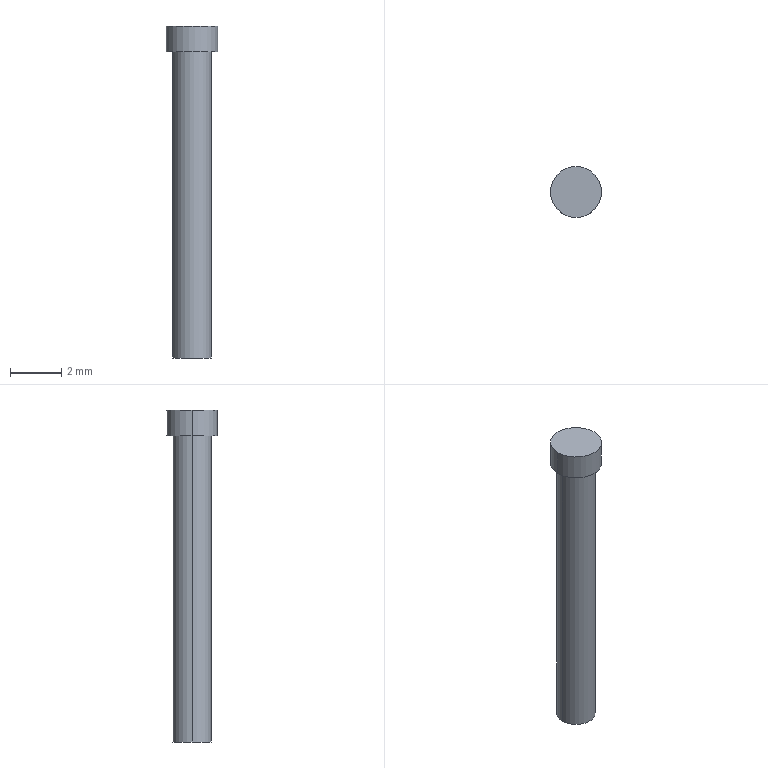Part | SolidWorks | features Extrusion 1, ICE 1 | 1 solid | 7 faces | box 2 x 2 x 13 mm | volume 24.347 mm3 | cylinder 4 | plane 3 | commonest cylinder face diameters 1.5 x2 2 x2
STEP:
#1=CARTESIAN_POINT('',(1.,0.,13.));
#2=VERTEX_POINT('',#1);
#3=CARTESIAN_POINT('',(-1.,0.,13.));
#4=VERTEX_POINT('',#3);
#5=CARTESIAN_POINT('',(0.,0.,13.));
#6=DIRECTION('',(0.,0.,1.));
#7=DIRECTION('',(1.,0.,0.));
#8=AXIS2_PLACEMENT_3D('',#5,#6,#7);
#9=CIRCLE('',#8,1.);
#10=EDGE_CURVE('',#2,#4,#9,.T.);
#11=ORIENTED_EDGE('',*,*,#10,.F.);
#12=CARTESIAN_POINT('',(1.,0.,12.));
#13=VERTEX_POINT('',#12);
#14=CARTESIAN_POINT('',(1.,0.,13.));
#15=DIRECTION('',(0.,0.,-1.));
#16=VECTOR('',#15,1000.);
#17=LINE('',#14,#16);
#18=EDGE_CURVE('',#2,#13,#17,.T.);
#19=ORIENTED_EDGE('',*,*,#18,.T.);
#20=CARTESIAN_POINT('',(-1.,0.,12.));
#21=VERTEX_POINT('',#20);
#22=CARTESIAN_POINT('',(0.,0.,12.));
#23=DIRECTION('',(0.,0.,1.));
#24=DIRECTION('',(1.,0.,0.));
#25=AXIS2_PLACEMENT_3D('',#22,#23,#24);
#26=CIRCLE('',#25,1.);
#27=EDGE_CURVE('',#13,#21,#26,.T.);
#28=ORIENTED_EDGE('',*,*,#27,.T.);
#29=CARTESIAN_POINT('',(-1.,0.,13.));
#30=DIRECTION('',(0.,0.,-1.));
#31=VECTOR('',#30,1000.);
#32=LINE('',#29,#31);
#33=EDGE_CURVE('',#4,#21,#32,.T.);
#34=ORIENTED_EDGE('',*,*,#33,.F.);
#35=EDGE_LOOP('',(#11,#19,#28,#34));
#36=FACE_OUTER_BOUND('',#35,.T.);
#37=CARTESIAN_POINT('',(0.,0.,13.));
#38=DIRECTION('',(0.,0.,-1.));
#39=DIRECTION('',(-1.,0.,0.));
#40=AXIS2_PLACEMENT_3D('',#37,#38,#39);
#41=CYLINDRICAL_SURFACE('',#40,1.);
#42=ADVANCED_FACE('',(#36),#41,.T.);
#43=CARTESIAN_POINT('',(0.75,0.,12.));
#44=VERTEX_POINT('',#43);
#45=CARTESIAN_POINT('',(-0.75,0.,12.));
#46=VERTEX_POINT('',#45);
#47=CARTESIAN_POINT('',(0.,0.,12.));
#48=DIRECTION('',(0.,0.,1.));
#49=DIRECTION('',(1.,0.,0.));
#50=AXIS2_PLACEMENT_3D('',#47,#48,#49);
#51=CIRCLE('',#50,0.75);
#52=EDGE_CURVE('',#44,#46,#51,.T.);
#53=ORIENTED_EDGE('',*,*,#52,.F.);
#54=CARTESIAN_POINT('',(0.75,0.,0.));
#55=VERTEX_POINT('',#54);
#56=CARTESIAN_POINT('',(0.75,0.,12.));
#57=DIRECTION('',(0.,0.,-1.));
#58=VECTOR('',#57,1000.);
#59=LINE('',#56,#58);
#60=EDGE_CURVE('',#44,#55,#59,.T.);
#61=ORIENTED_EDGE('',*,*,#60,.T.);
#62=CARTESIAN_POINT('',(-0.75,0.,0.));
#63=VERTEX_POINT('',#62);
#64=CARTESIAN_POINT('',(0.,0.,0.));
#65=DIRECTION('',(0.,0.,1.));
#66=DIRECTION('',(1.,0.,0.));
#67=AXIS2_PLACEMENT_3D('',#64,#65,#66);
#68=CIRCLE('',#67,0.75);
#69=EDGE_CURVE('',#55,#63,#68,.T.);
#70=ORIENTED_EDGE('',*,*,#69,.T.);
#71=CARTESIAN_POINT('',(-0.75,0.,12.));
#72=DIRECTION('',(0.,0.,-1.));
#73=VECTOR('',#72,1000.);
#74=LINE('',#71,#73);
#75=EDGE_CURVE('',#46,#63,#74,.T.);
#76=ORIENTED_EDGE('',*,*,#75,.F.);
#77=EDGE_LOOP('',(#53,#61,#70,#76));
#78=FACE_OUTER_BOUND('',#77,.T.);
#79=CARTESIAN_POINT('',(0.,0.,12.));
#80=DIRECTION('',(0.,0.,-1.));
#81=DIRECTION('',(-1.,0.,0.));
#82=AXIS2_PLACEMENT_3D('',#79,#80,#81);
#83=CYLINDRICAL_SURFACE('',#82,0.75);
#84=ADVANCED_FACE('',(#78),#83,.T.);
#85=ORIENTED_EDGE('',*,*,#60,.F.);
#86=CARTESIAN_POINT('',(0.,0.,12.));
#87=DIRECTION('',(0.,0.,1.));
#88=DIRECTION('',(1.,0.,0.));
#89=AXIS2_PLACEMENT_3D('',#86,#87,#88);
#90=CIRCLE('',#89,0.75);
#91=EDGE_CURVE('',#46,#44,#90,.T.);
#92=ORIENTED_EDGE('',*,*,#91,.F.);
#93=ORIENTED_EDGE('',*,*,#75,.T.);
#94=CARTESIAN_POINT('',(0.,0.,0.));
#95=DIRECTION('',(0.,0.,1.));
#96=DIRECTION('',(1.,0.,0.));
#97=AXIS2_PLACEMENT_3D('',#94,#95,#96);
#98=CIRCLE('',#97,0.75);
#99=EDGE_CURVE('',#63,#55,#98,.T.);
#100=ORIENTED_EDGE('',*,*,#99,.T.);
#101=EDGE_LOOP('',(#85,#92,#93,#100));
#102=FACE_OUTER_BOUND('',#101,.T.);
#103=CARTESIAN_POINT('',(0.,0.,12.));
#104=DIRECTION('',(0.,0.,-1.));
#105=DIRECTION('',(-1.,0.,0.));
#106=AXIS2_PLACEMENT_3D('',#103,#104,#105);
#107=CYLINDRICAL_SURFACE('',#106,0.75);
#108=ADVANCED_FACE('',(#102),#107,.T.);
#109=ORIENTED_EDGE('',*,*,#99,.F.);
#110=ORIENTED_EDGE('',*,*,#69,.F.);
#111=EDGE_LOOP('',(#109,#110));
#112=FACE_OUTER_BOUND('',#111,.T.);
#113=CARTESIAN_POINT('',(0.,0.,0.));
#114=DIRECTION('',(0.,0.,1.));
#115=DIRECTION('',(1.,0.,0.));
#116=AXIS2_PLACEMENT_3D('',#113,#114,#115);
#117=PLANE('',#116);
#118=ADVANCED_FACE('',(#112),#117,.F.);
#119=ORIENTED_EDGE('',*,*,#18,.F.);
#120=CARTESIAN_POINT('',(0.,0.,13.));
#121=DIRECTION('',(0.,0.,1.));
#122=DIRECTION('',(1.,0.,0.));
#123=AXIS2_PLACEMENT_3D('',#120,#121,#122);
#124=CIRCLE('',#123,1.);
#125=EDGE_CURVE('',#4,#2,#124,.T.);
#126=ORIENTED_EDGE('',*,*,#125,.F.);
#127=ORIENTED_EDGE('',*,*,#33,.T.);
#128=CARTESIAN_POINT('',(0.,0.,12.));
#129=DIRECTION('',(0.,0.,1.));
#130=DIRECTION('',(1.,0.,0.));
#131=AXIS2_PLACEMENT_3D('',#128,#129,#130);
#132=CIRCLE('',#131,1.);
#133=EDGE_CURVE('',#21,#13,#132,.T.);
#134=ORIENTED_EDGE('',*,*,#133,.T.);
#135=EDGE_LOOP('',(#119,#126,#127,#134));
#136=FACE_OUTER_BOUND('',#135,.T.);
#137=CARTESIAN_POINT('',(0.,0.,13.));
#138=DIRECTION('',(0.,0.,-1.));
#139=DIRECTION('',(-1.,0.,0.));
#140=AXIS2_PLACEMENT_3D('',#137,#138,#139);
#141=CYLINDRICAL_SURFACE('',#140,1.);
#142=ADVANCED_FACE('',(#136),#141,.T.);
#143=ORIENTED_EDGE('',*,*,#125,.T.);
#144=ORIENTED_EDGE('',*,*,#10,.T.);
#145=EDGE_LOOP('',(#143,#144));
#146=FACE_OUTER_BOUND('',#145,.T.);
#147=CARTESIAN_POINT('',(0.,0.,13.));
#148=DIRECTION('',(0.,0.,1.));
#149=DIRECTION('',(1.,0.,0.));
#150=AXIS2_PLACEMENT_3D('',#147,#148,#149);
#151=PLANE('',#150);
#152=ADVANCED_FACE('',(#146),#151,.T.);
#153=ORIENTED_EDGE('',*,*,#91,.T.);
#154=ORIENTED_EDGE('',*,*,#52,.T.);
#155=EDGE_LOOP('',(#153,#154));
#156=FACE_BOUND('',#155,.T.);
#157=ORIENTED_EDGE('',*,*,#133,.F.);
#158=ORIENTED_EDGE('',*,*,#27,.F.);
#159=EDGE_LOOP('',(#157,#158));
#160=FACE_OUTER_BOUND('',#159,.T.);
#161=CARTESIAN_POINT('',(0.,0.,12.));
#162=DIRECTION('',(0.,0.,1.));
#163=DIRECTION('',(1.,0.,0.));
#164=AXIS2_PLACEMENT_3D('',#161,#162,#163);
#165=PLANE('',#164);
#166=ADVANCED_FACE('',(#156,#160),#165,.F.);
#167=CLOSED_SHELL('',(#42,#84,#108,#118,#142,#152,#166));
#168=MANIFOLD_SOLID_BREP('',#167);
#169=CARTESIAN_POINT('',(0.,0.,0.));
#170=DIRECTION('',(0.,0.,1.));
#171=DIRECTION('',(1.,0.,0.));
#172=AXIS2_PLACEMENT_3D('',#169,#170,#171);
#173=(LENGTH_UNIT()NAMED_UNIT(*)SI_UNIT(.MILLI.,.METRE.));
#174=UNCERTAINTY_MEASURE_WITH_UNIT(LENGTH_MEASURE(0.00001),#173,'','');
#175=(NAMED_UNIT(*)PLANE_ANGLE_UNIT()SI_UNIT($,.RADIAN.));
#176=(NAMED_UNIT(*)SI_UNIT($,.STERADIAN.)SOLID_ANGLE_UNIT());
#177=(GEOMETRIC_REPRESENTATION_CONTEXT(3)GLOBAL_UNCERTAINTY_ASSIGNED_CONTEXT((#174))GLOBAL_UNIT_ASSIGNED_CONTEXT((#173,#175,#176))REPRESENTATION_CONTEXT('',''));
#178=ADVANCED_BREP_SHAPE_REPRESENTATION('',(#168,#172),#177);